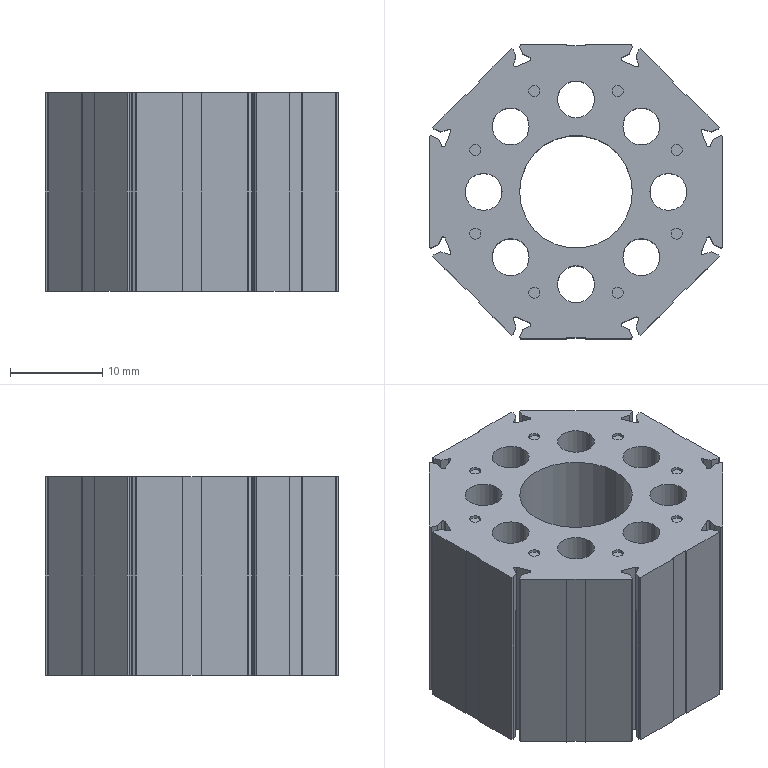Part | STEP file | TQ-DD-1105-THRotorCore1010_デフォルト | 1 solid | 186 faces | box 31.8 x 31.8 x 21.5 mm | volume 12871 mm3 | plane 114 | cylinder 72 | commonest cylinder face diameters 1.2 x32 0.4 x22 4 x16 12.2 x2